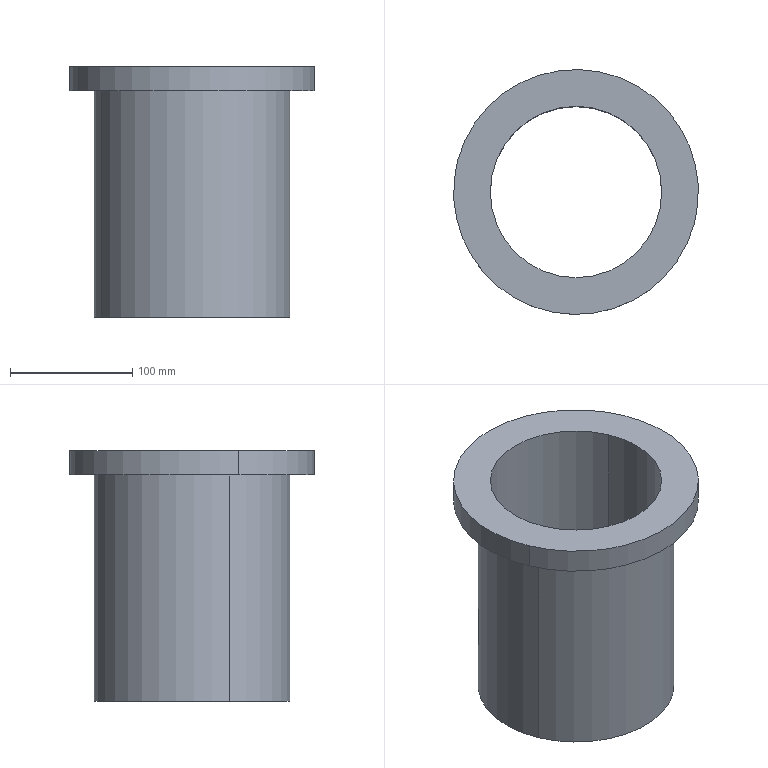Part | SolidWorks | features BaseBody 1 | 1 solid | 9 faces | box 200 x 200 x 205 mm | volume 1192234 mm3 | cylinder 6 | plane 3 | commonest cylinder face diameters 140 x2 160 x2 200 x2
STEP:
#1=CARTESIAN_POINT('',(329.738,980.062,405.107));
#2=VERTEX_POINT('',#1);
#3=CARTESIAN_POINT('',(200.416,926.436,405.107));
#4=VERTEX_POINT('',#3);
#5=CARTESIAN_POINT('',(265.077,953.249,405.107));
#6=DIRECTION('',(0.,0.,-1.));
#7=DIRECTION('',(-0.9237,-0.383,0.));
#8=AXIS2_PLACEMENT_3D('',#5,#6,#7);
#9=CIRCLE('',#8,70.);
#10=EDGE_CURVE('',#2,#4,#9,.T.);
#11=ORIENTED_EDGE('',*,*,#10,.F.);
#12=CARTESIAN_POINT('',(265.077,953.249,405.107));
#13=DIRECTION('',(0.,0.,-1.));
#14=DIRECTION('',(-0.9237,-0.383,0.));
#15=AXIS2_PLACEMENT_3D('',#12,#13,#14);
#16=CIRCLE('',#15,70.);
#17=EDGE_CURVE('',#4,#2,#16,.T.);
#18=ORIENTED_EDGE('',*,*,#17,.F.);
#19=EDGE_LOOP('',(#11,#18));
#20=FACE_BOUND('',#19,.T.);
#21=CARTESIAN_POINT('',(338.975,983.893,405.107));
#22=VERTEX_POINT('',#21);
#23=CARTESIAN_POINT('',(191.179,922.605,405.107));
#24=VERTEX_POINT('',#23);
#25=CARTESIAN_POINT('',(265.077,953.249,405.107));
#26=DIRECTION('',(0.,0.,-1.));
#27=DIRECTION('',(-0.9237,-0.383,0.));
#28=AXIS2_PLACEMENT_3D('',#25,#26,#27);
#29=CIRCLE('',#28,80.);
#30=EDGE_CURVE('',#22,#24,#29,.T.);
#31=ORIENTED_EDGE('',*,*,#30,.T.);
#32=CARTESIAN_POINT('',(265.077,953.249,405.107));
#33=DIRECTION('',(0.,0.,-1.));
#34=DIRECTION('',(-0.9237,-0.383,0.));
#35=AXIS2_PLACEMENT_3D('',#32,#33,#34);
#36=CIRCLE('',#35,80.);
#37=EDGE_CURVE('',#24,#22,#36,.T.);
#38=ORIENTED_EDGE('',*,*,#37,.T.);
#39=EDGE_LOOP('',(#31,#38));
#40=FACE_OUTER_BOUND('',#39,.T.);
#41=CARTESIAN_POINT('',(265.077,953.249,405.107));
#42=DIRECTION('',(0.,0.,-1.));
#43=DIRECTION('',(0.,-1.,0.));
#44=AXIS2_PLACEMENT_3D('',#41,#42,#43);
#45=PLANE('',#44);
#46=ADVANCED_FACE('',(#20,#40),#45,.T.);
#47=CARTESIAN_POINT('',(172.704,914.944,610.107));
#48=VERTEX_POINT('',#47);
#49=CARTESIAN_POINT('',(172.704,914.944,590.107));
#50=VERTEX_POINT('',#49);
#51=CARTESIAN_POINT('',(172.704,914.944,590.107));
#52=DIRECTION('',(0.,0.,-1.));
#53=VECTOR('',#52,1000.);
#54=LINE('',#51,#53);
#55=EDGE_CURVE('',#48,#50,#54,.T.);
#56=ORIENTED_EDGE('',*,*,#55,.T.);
#57=CARTESIAN_POINT('',(357.45,991.554,590.107));
#58=VERTEX_POINT('',#57);
#59=CARTESIAN_POINT('',(265.077,953.249,590.107));
#60=DIRECTION('',(0.,0.,-1.));
#61=DIRECTION('',(-0.9237,-0.383,0.));
#62=AXIS2_PLACEMENT_3D('',#59,#60,#61);
#63=CIRCLE('',#62,100.);
#64=EDGE_CURVE('',#58,#50,#63,.T.);
#65=ORIENTED_EDGE('',*,*,#64,.F.);
#66=CARTESIAN_POINT('',(357.45,991.554,610.107));
#67=VERTEX_POINT('',#66);
#68=CARTESIAN_POINT('',(357.45,991.554,590.107));
#69=DIRECTION('',(0.,0.,-1.));
#70=VECTOR('',#69,1000.);
#71=LINE('',#68,#70);
#72=EDGE_CURVE('',#67,#58,#71,.T.);
#73=ORIENTED_EDGE('',*,*,#72,.F.);
#74=CARTESIAN_POINT('',(265.077,953.249,610.107));
#75=DIRECTION('',(0.,0.,-1.));
#76=DIRECTION('',(-0.9237,-0.383,0.));
#77=AXIS2_PLACEMENT_3D('',#74,#75,#76);
#78=CIRCLE('',#77,100.);
#79=EDGE_CURVE('',#67,#48,#78,.T.);
#80=ORIENTED_EDGE('',*,*,#79,.T.);
#81=EDGE_LOOP('',(#56,#65,#73,#80));
#82=FACE_OUTER_BOUND('',#81,.T.);
#83=CARTESIAN_POINT('',(265.077,953.249,590.107));
#84=DIRECTION('',(0.,0.,1.));
#85=DIRECTION('',(-0.9237,-0.383,0.));
#86=AXIS2_PLACEMENT_3D('',#83,#84,#85);
#87=CYLINDRICAL_SURFACE('',#86,100.);
#88=ADVANCED_FACE('',(#82),#87,.T.);
#89=CARTESIAN_POINT('',(338.975,983.893,590.107));
#90=VERTEX_POINT('',#89);
#91=CARTESIAN_POINT('',(191.179,922.605,590.107));
#92=VERTEX_POINT('',#91);
#93=CARTESIAN_POINT('',(265.077,953.249,590.107));
#94=DIRECTION('',(0.,0.,1.));
#95=DIRECTION('',(-0.9237,-0.383,0.));
#96=AXIS2_PLACEMENT_3D('',#93,#94,#95);
#97=CIRCLE('',#96,80.);
#98=EDGE_CURVE('',#90,#92,#97,.T.);
#99=ORIENTED_EDGE('',*,*,#98,.T.);
#100=CARTESIAN_POINT('',(265.077,953.249,590.107));
#101=DIRECTION('',(0.,0.,1.));
#102=DIRECTION('',(-0.9237,-0.383,0.));
#103=AXIS2_PLACEMENT_3D('',#100,#101,#102);
#104=CIRCLE('',#103,80.);
#105=EDGE_CURVE('',#92,#90,#104,.T.);
#106=ORIENTED_EDGE('',*,*,#105,.T.);
#107=EDGE_LOOP('',(#99,#106));
#108=FACE_BOUND('',#107,.T.);
#109=ORIENTED_EDGE('',*,*,#64,.T.);
#110=CARTESIAN_POINT('',(265.077,953.249,590.107));
#111=DIRECTION('',(0.,0.,-1.));
#112=DIRECTION('',(-0.9237,-0.383,0.));
#113=AXIS2_PLACEMENT_3D('',#110,#111,#112);
#114=CIRCLE('',#113,100.);
#115=EDGE_CURVE('',#50,#58,#114,.T.);
#116=ORIENTED_EDGE('',*,*,#115,.T.);
#117=EDGE_LOOP('',(#109,#116));
#118=FACE_OUTER_BOUND('',#117,.T.);
#119=CARTESIAN_POINT('',(265.077,953.249,590.107));
#120=DIRECTION('',(0.,0.,-1.));
#121=DIRECTION('',(0.,-1.,0.));
#122=AXIS2_PLACEMENT_3D('',#119,#120,#121);
#123=PLANE('',#122);
#124=ADVANCED_FACE('',(#108,#118),#123,.T.);
#125=CARTESIAN_POINT('',(329.738,980.062,610.107));
#126=VERTEX_POINT('',#125);
#127=CARTESIAN_POINT('',(200.416,926.436,610.107));
#128=VERTEX_POINT('',#127);
#129=CARTESIAN_POINT('',(265.077,953.249,610.107));
#130=DIRECTION('',(0.,0.,-1.));
#131=DIRECTION('',(-0.9237,-0.383,0.));
#132=AXIS2_PLACEMENT_3D('',#129,#130,#131);
#133=CIRCLE('',#132,70.);
#134=EDGE_CURVE('',#126,#128,#133,.T.);
#135=ORIENTED_EDGE('',*,*,#134,.T.);
#136=CARTESIAN_POINT('',(265.077,953.249,610.107));
#137=DIRECTION('',(0.,0.,-1.));
#138=DIRECTION('',(-0.9237,-0.383,0.));
#139=AXIS2_PLACEMENT_3D('',#136,#137,#138);
#140=CIRCLE('',#139,70.);
#141=EDGE_CURVE('',#128,#126,#140,.T.);
#142=ORIENTED_EDGE('',*,*,#141,.T.);
#143=EDGE_LOOP('',(#135,#142));
#144=FACE_BOUND('',#143,.T.);
#145=ORIENTED_EDGE('',*,*,#79,.F.);
#146=CARTESIAN_POINT('',(265.077,953.249,610.107));
#147=DIRECTION('',(0.,0.,-1.));
#148=DIRECTION('',(-0.9237,-0.383,0.));
#149=AXIS2_PLACEMENT_3D('',#146,#147,#148);
#150=CIRCLE('',#149,100.);
#151=EDGE_CURVE('',#48,#67,#150,.T.);
#152=ORIENTED_EDGE('',*,*,#151,.F.);
#153=EDGE_LOOP('',(#145,#152));
#154=FACE_OUTER_BOUND('',#153,.T.);
#155=CARTESIAN_POINT('',(265.077,953.249,610.107));
#156=DIRECTION('',(0.,0.,-1.));
#157=DIRECTION('',(0.,-1.,0.));
#158=AXIS2_PLACEMENT_3D('',#155,#156,#157);
#159=PLANE('',#158);
#160=ADVANCED_FACE('',(#144,#154),#159,.F.);
#161=ORIENTED_EDGE('',*,*,#115,.F.);
#162=ORIENTED_EDGE('',*,*,#55,.F.);
#163=ORIENTED_EDGE('',*,*,#151,.T.);
#164=ORIENTED_EDGE('',*,*,#72,.T.);
#165=EDGE_LOOP('',(#161,#162,#163,#164));
#166=FACE_OUTER_BOUND('',#165,.T.);
#167=CARTESIAN_POINT('',(265.077,953.249,590.107));
#168=DIRECTION('',(0.,0.,1.));
#169=DIRECTION('',(-0.9237,-0.383,0.));
#170=AXIS2_PLACEMENT_3D('',#167,#168,#169);
#171=CYLINDRICAL_SURFACE('',#170,100.);
#172=ADVANCED_FACE('',(#166),#171,.T.);
#173=CARTESIAN_POINT('',(200.416,926.436,355.107));
#174=DIRECTION('',(0.,0.,-1.));
#175=VECTOR('',#174,1000.);
#176=LINE('',#173,#175);
#177=EDGE_CURVE('',#128,#4,#176,.T.);
#178=ORIENTED_EDGE('',*,*,#177,.T.);
#179=ORIENTED_EDGE('',*,*,#17,.T.);
#180=CARTESIAN_POINT('',(329.738,980.062,355.107));
#181=DIRECTION('',(0.,0.,-1.));
#182=VECTOR('',#181,1000.);
#183=LINE('',#180,#182);
#184=EDGE_CURVE('',#126,#2,#183,.T.);
#185=ORIENTED_EDGE('',*,*,#184,.F.);
#186=ORIENTED_EDGE('',*,*,#141,.F.);
#187=EDGE_LOOP('',(#178,#179,#185,#186));
#188=FACE_OUTER_BOUND('',#187,.T.);
#189=CARTESIAN_POINT('',(265.077,953.249,355.107));
#190=DIRECTION('',(0.,0.,1.));
#191=DIRECTION('',(-0.9237,-0.383,0.));
#192=AXIS2_PLACEMENT_3D('',#189,#190,#191);
#193=CYLINDRICAL_SURFACE('',#192,70.);
#194=ADVANCED_FACE('',(#188),#193,.F.);
#195=CARTESIAN_POINT('',(191.179,922.605,355.107));
#196=DIRECTION('',(0.,0.,-1.));
#197=VECTOR('',#196,1000.);
#198=LINE('',#195,#197);
#199=EDGE_CURVE('',#92,#24,#198,.T.);
#200=ORIENTED_EDGE('',*,*,#199,.T.);
#201=ORIENTED_EDGE('',*,*,#30,.F.);
#202=CARTESIAN_POINT('',(338.975,983.893,355.107));
#203=DIRECTION('',(0.,0.,-1.));
#204=VECTOR('',#203,1000.);
#205=LINE('',#202,#204);
#206=EDGE_CURVE('',#90,#22,#205,.T.);
#207=ORIENTED_EDGE('',*,*,#206,.F.);
#208=ORIENTED_EDGE('',*,*,#105,.F.);
#209=EDGE_LOOP('',(#200,#201,#207,#208));
#210=FACE_OUTER_BOUND('',#209,.T.);
#211=CARTESIAN_POINT('',(265.077,953.249,355.107));
#212=DIRECTION('',(0.,0.,1.));
#213=DIRECTION('',(-0.9237,-0.383,0.));
#214=AXIS2_PLACEMENT_3D('',#211,#212,#213);
#215=CYLINDRICAL_SURFACE('',#214,80.);
#216=ADVANCED_FACE('',(#210),#215,.T.);
#217=ORIENTED_EDGE('',*,*,#206,.T.);
#218=ORIENTED_EDGE('',*,*,#37,.F.);
#219=ORIENTED_EDGE('',*,*,#199,.F.);
#220=ORIENTED_EDGE('',*,*,#98,.F.);
#221=EDGE_LOOP('',(#217,#218,#219,#220));
#222=FACE_OUTER_BOUND('',#221,.T.);
#223=CARTESIAN_POINT('',(265.077,953.249,355.107));
#224=DIRECTION('',(0.,0.,1.));
#225=DIRECTION('',(-0.9237,-0.383,0.));
#226=AXIS2_PLACEMENT_3D('',#223,#224,#225);
#227=CYLINDRICAL_SURFACE('',#226,80.);
#228=ADVANCED_FACE('',(#222),#227,.T.);
#229=ORIENTED_EDGE('',*,*,#184,.T.);
#230=ORIENTED_EDGE('',*,*,#10,.T.);
#231=ORIENTED_EDGE('',*,*,#177,.F.);
#232=ORIENTED_EDGE('',*,*,#134,.F.);
#233=EDGE_LOOP('',(#229,#230,#231,#232));
#234=FACE_OUTER_BOUND('',#233,.T.);
#235=CARTESIAN_POINT('',(265.077,953.249,355.107));
#236=DIRECTION('',(0.,0.,1.));
#237=DIRECTION('',(-0.9237,-0.383,0.));
#238=AXIS2_PLACEMENT_3D('',#235,#236,#237);
#239=CYLINDRICAL_SURFACE('',#238,70.);
#240=ADVANCED_FACE('',(#234),#239,.F.);
#241=CLOSED_SHELL('',(#46,#88,#124,#160,#172,#194,#216,#228,#240));
#242=MANIFOLD_SOLID_BREP('',#241);
#243=CARTESIAN_POINT('',(0.,0.,0.));
#244=DIRECTION('',(0.,0.,1.));
#245=DIRECTION('',(1.,0.,0.));
#246=AXIS2_PLACEMENT_3D('',#243,#244,#245);
#247=(LENGTH_UNIT()NAMED_UNIT(*)SI_UNIT(.MILLI.,.METRE.));
#248=UNCERTAINTY_MEASURE_WITH_UNIT(LENGTH_MEASURE(0.00001),#247,'','');
#249=(NAMED_UNIT(*)PLANE_ANGLE_UNIT()SI_UNIT($,.RADIAN.));
#250=(NAMED_UNIT(*)SI_UNIT($,.STERADIAN.)SOLID_ANGLE_UNIT());
#251=(GEOMETRIC_REPRESENTATION_CONTEXT(3)GLOBAL_UNCERTAINTY_ASSIGNED_CONTEXT((#248))GLOBAL_UNIT_ASSIGNED_CONTEXT((#247,#249,#250))REPRESENTATION_CONTEXT('',''));
#252=ADVANCED_BREP_SHAPE_REPRESENTATION('',(#242,#246),#251);